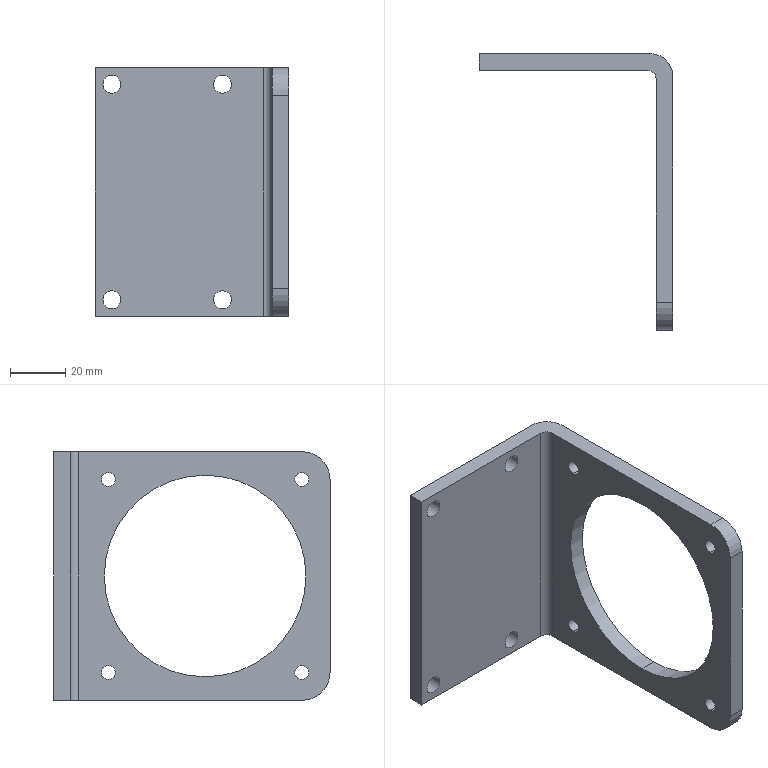Part | STEP file | X77-04015 | 1 solid | 30 faces | box 70 x 100 x 90 mm | volume 60860 mm3 | cylinder 22 | plane 8 | commonest cylinder face diameters 5 x8 6.5 x8 20 x2 73 x2 6 x1 16 x1
STEP:
#1=CARTESIAN_POINT('',(364.189,-105.641,7.5));
#2=VERTEX_POINT('',#1);
#3=CARTESIAN_POINT('',(364.189,-105.641,12.5));
#4=VERTEX_POINT('',#3);
#5=CARTESIAN_POINT('',(364.189,-105.641,10.));
#6=DIRECTION('',(-1.,0.,0.));
#7=DIRECTION('',(0.,0.,1.));
#8=AXIS2_PLACEMENT_3D('',#5,#6,#7);
#9=CIRCLE('',#8,2.5);
#10=EDGE_CURVE('',#2,#4,#9,.T.);
#11=ORIENTED_EDGE('',*,*,#10,.F.);
#12=CARTESIAN_POINT('',(358.189,-105.641,7.5));
#13=VERTEX_POINT('',#12);
#14=CARTESIAN_POINT('',(358.189,-105.641,7.5));
#15=DIRECTION('',(-1.,0.,0.));
#16=VECTOR('',#15,1000.);
#17=LINE('',#14,#16);
#18=EDGE_CURVE('',#2,#13,#17,.T.);
#19=ORIENTED_EDGE('',*,*,#18,.T.);
#20=CARTESIAN_POINT('',(358.189,-105.641,12.5));
#21=VERTEX_POINT('',#20);
#22=CARTESIAN_POINT('',(358.189,-105.641,10.));
#23=DIRECTION('',(-1.,0.,0.));
#24=DIRECTION('',(0.,0.,1.));
#25=AXIS2_PLACEMENT_3D('',#22,#23,#24);
#26=CIRCLE('',#25,2.5);
#27=EDGE_CURVE('',#13,#21,#26,.T.);
#28=ORIENTED_EDGE('',*,*,#27,.T.);
#29=CARTESIAN_POINT('',(358.189,-105.641,12.5));
#30=DIRECTION('',(-1.,0.,0.));
#31=VECTOR('',#30,1000.);
#32=LINE('',#29,#31);
#33=EDGE_CURVE('',#4,#21,#32,.T.);
#34=ORIENTED_EDGE('',*,*,#33,.F.);
#35=EDGE_LOOP('',(#11,#19,#28,#34));
#36=FACE_OUTER_BOUND('',#35,.T.);
#37=CARTESIAN_POINT('',(358.189,-105.641,10.));
#38=DIRECTION('',(-1.,0.,0.));
#39=DIRECTION('',(0.,0.,1.));
#40=AXIS2_PLACEMENT_3D('',#37,#38,#39);
#41=CYLINDRICAL_SURFACE('',#40,2.5);
#42=ADVANCED_FACE('',(#36),#41,.F.);
#43=CARTESIAN_POINT('',(364.189,-105.641,77.5));
#44=VERTEX_POINT('',#43);
#45=CARTESIAN_POINT('',(364.189,-105.641,82.5));
#46=VERTEX_POINT('',#45);
#47=CARTESIAN_POINT('',(364.189,-105.641,80.));
#48=DIRECTION('',(-1.,0.,0.));
#49=DIRECTION('',(0.,0.,1.));
#50=AXIS2_PLACEMENT_3D('',#47,#48,#49);
#51=CIRCLE('',#50,2.5);
#52=EDGE_CURVE('',#44,#46,#51,.T.);
#53=ORIENTED_EDGE('',*,*,#52,.F.);
#54=CARTESIAN_POINT('',(358.189,-105.641,77.5));
#55=VERTEX_POINT('',#54);
#56=CARTESIAN_POINT('',(358.189,-105.641,77.5));
#57=DIRECTION('',(-1.,0.,0.));
#58=VECTOR('',#57,1000.);
#59=LINE('',#56,#58);
#60=EDGE_CURVE('',#44,#55,#59,.T.);
#61=ORIENTED_EDGE('',*,*,#60,.T.);
#62=CARTESIAN_POINT('',(358.189,-105.641,82.5));
#63=VERTEX_POINT('',#62);
#64=CARTESIAN_POINT('',(358.189,-105.641,80.));
#65=DIRECTION('',(-1.,0.,0.));
#66=DIRECTION('',(0.,0.,1.));
#67=AXIS2_PLACEMENT_3D('',#64,#65,#66);
#68=CIRCLE('',#67,2.5);
#69=EDGE_CURVE('',#55,#63,#68,.T.);
#70=ORIENTED_EDGE('',*,*,#69,.T.);
#71=CARTESIAN_POINT('',(358.189,-105.641,82.5));
#72=DIRECTION('',(-1.,0.,0.));
#73=VECTOR('',#72,1000.);
#74=LINE('',#71,#73);
#75=EDGE_CURVE('',#46,#63,#74,.T.);
#76=ORIENTED_EDGE('',*,*,#75,.F.);
#77=EDGE_LOOP('',(#53,#61,#70,#76));
#78=FACE_OUTER_BOUND('',#77,.T.);
#79=CARTESIAN_POINT('',(358.189,-105.641,80.));
#80=DIRECTION('',(-1.,0.,0.));
#81=DIRECTION('',(0.,0.,1.));
#82=AXIS2_PLACEMENT_3D('',#79,#80,#81);
#83=CYLINDRICAL_SURFACE('',#82,2.5);
#84=ADVANCED_FACE('',(#78),#83,.F.);
#85=CARTESIAN_POINT('',(364.189,-35.641,77.5));
#86=VERTEX_POINT('',#85);
#87=CARTESIAN_POINT('',(364.189,-35.641,82.5));
#88=VERTEX_POINT('',#87);
#89=CARTESIAN_POINT('',(364.189,-35.641,80.));
#90=DIRECTION('',(-1.,0.,0.));
#91=DIRECTION('',(0.,0.,1.));
#92=AXIS2_PLACEMENT_3D('',#89,#90,#91);
#93=CIRCLE('',#92,2.5);
#94=EDGE_CURVE('',#86,#88,#93,.T.);
#95=ORIENTED_EDGE('',*,*,#94,.F.);
#96=CARTESIAN_POINT('',(358.189,-35.641,77.5));
#97=VERTEX_POINT('',#96);
#98=CARTESIAN_POINT('',(358.189,-35.641,77.5));
#99=DIRECTION('',(-1.,0.,0.));
#100=VECTOR('',#99,1000.);
#101=LINE('',#98,#100);
#102=EDGE_CURVE('',#86,#97,#101,.T.);
#103=ORIENTED_EDGE('',*,*,#102,.T.);
#104=CARTESIAN_POINT('',(358.189,-35.641,82.5));
#105=VERTEX_POINT('',#104);
#106=CARTESIAN_POINT('',(358.189,-35.641,80.));
#107=DIRECTION('',(-1.,0.,0.));
#108=DIRECTION('',(0.,0.,1.));
#109=AXIS2_PLACEMENT_3D('',#106,#107,#108);
#110=CIRCLE('',#109,2.5);
#111=EDGE_CURVE('',#97,#105,#110,.T.);
#112=ORIENTED_EDGE('',*,*,#111,.T.);
#113=CARTESIAN_POINT('',(358.189,-35.641,82.5));
#114=DIRECTION('',(-1.,0.,0.));
#115=VECTOR('',#114,1000.);
#116=LINE('',#113,#115);
#117=EDGE_CURVE('',#88,#105,#116,.T.);
#118=ORIENTED_EDGE('',*,*,#117,.F.);
#119=EDGE_LOOP('',(#95,#103,#112,#118));
#120=FACE_OUTER_BOUND('',#119,.T.);
#121=CARTESIAN_POINT('',(358.189,-35.641,80.));
#122=DIRECTION('',(-1.,0.,0.));
#123=DIRECTION('',(0.,0.,1.));
#124=AXIS2_PLACEMENT_3D('',#121,#122,#123);
#125=CYLINDRICAL_SURFACE('',#124,2.5);
#126=ADVANCED_FACE('',(#120),#125,.F.);
#127=CARTESIAN_POINT('',(364.189,-35.641,7.5));
#128=VERTEX_POINT('',#127);
#129=CARTESIAN_POINT('',(364.189,-35.641,12.5));
#130=VERTEX_POINT('',#129);
#131=CARTESIAN_POINT('',(364.189,-35.641,10.));
#132=DIRECTION('',(-1.,0.,0.));
#133=DIRECTION('',(0.,0.,1.));
#134=AXIS2_PLACEMENT_3D('',#131,#132,#133);
#135=CIRCLE('',#134,2.5);
#136=EDGE_CURVE('',#128,#130,#135,.T.);
#137=ORIENTED_EDGE('',*,*,#136,.F.);
#138=CARTESIAN_POINT('',(358.189,-35.641,7.5));
#139=VERTEX_POINT('',#138);
#140=CARTESIAN_POINT('',(358.189,-35.641,7.5));
#141=DIRECTION('',(-1.,0.,0.));
#142=VECTOR('',#141,1000.);
#143=LINE('',#140,#142);
#144=EDGE_CURVE('',#128,#139,#143,.T.);
#145=ORIENTED_EDGE('',*,*,#144,.T.);
#146=CARTESIAN_POINT('',(358.189,-35.641,12.5));
#147=VERTEX_POINT('',#146);
#148=CARTESIAN_POINT('',(358.189,-35.641,10.));
#149=DIRECTION('',(-1.,0.,0.));
#150=DIRECTION('',(0.,0.,1.));
#151=AXIS2_PLACEMENT_3D('',#148,#149,#150);
#152=CIRCLE('',#151,2.5);
#153=EDGE_CURVE('',#139,#147,#152,.T.);
#154=ORIENTED_EDGE('',*,*,#153,.T.);
#155=CARTESIAN_POINT('',(358.189,-35.641,12.5));
#156=DIRECTION('',(-1.,0.,0.));
#157=VECTOR('',#156,1000.);
#158=LINE('',#155,#157);
#159=EDGE_CURVE('',#130,#147,#158,.T.);
#160=ORIENTED_EDGE('',*,*,#159,.F.);
#161=EDGE_LOOP('',(#137,#145,#154,#160));
#162=FACE_OUTER_BOUND('',#161,.T.);
#163=CARTESIAN_POINT('',(358.189,-35.641,10.));
#164=DIRECTION('',(-1.,0.,0.));
#165=DIRECTION('',(0.,0.,1.));
#166=AXIS2_PLACEMENT_3D('',#163,#164,#165);
#167=CYLINDRICAL_SURFACE('',#166,2.5);
#168=ADVANCED_FACE('',(#162),#167,.F.);
#169=CARTESIAN_POINT('',(296.939,-15.891,6.));
#170=VERTEX_POINT('',#169);
#171=CARTESIAN_POINT('',(303.439,-15.891,6.));
#172=VERTEX_POINT('',#171);
#173=CARTESIAN_POINT('',(300.189,-15.891,6.));
#174=DIRECTION('',(0.,-1.,0.));
#175=DIRECTION('',(0.,0.,-1.));
#176=AXIS2_PLACEMENT_3D('',#173,#174,#175);
#177=CIRCLE('',#176,3.25);
#178=EDGE_CURVE('',#170,#172,#177,.T.);
#179=ORIENTED_EDGE('',*,*,#178,.F.);
#180=CARTESIAN_POINT('',(296.939,-21.891,6.));
#181=VERTEX_POINT('',#180);
#182=CARTESIAN_POINT('',(296.939,-11.891,6.));
#183=DIRECTION('',(0.,-1.,0.));
#184=VECTOR('',#183,1000.);
#185=LINE('',#182,#184);
#186=EDGE_CURVE('',#170,#181,#185,.T.);
#187=ORIENTED_EDGE('',*,*,#186,.T.);
#188=CARTESIAN_POINT('',(303.439,-21.891,6.));
#189=VERTEX_POINT('',#188);
#190=CARTESIAN_POINT('',(300.189,-21.891,6.));
#191=DIRECTION('',(0.,-1.,0.));
#192=DIRECTION('',(1.,0.,0.));
#193=AXIS2_PLACEMENT_3D('',#190,#191,#192);
#194=CIRCLE('',#193,3.25);
#195=EDGE_CURVE('',#181,#189,#194,.T.);
#196=ORIENTED_EDGE('',*,*,#195,.T.);
#197=CARTESIAN_POINT('',(303.439,-11.891,6.));
#198=DIRECTION('',(0.,-1.,0.));
#199=VECTOR('',#198,1000.);
#200=LINE('',#197,#199);
#201=EDGE_CURVE('',#172,#189,#200,.T.);
#202=ORIENTED_EDGE('',*,*,#201,.F.);
#203=EDGE_LOOP('',(#179,#187,#196,#202));
#204=FACE_OUTER_BOUND('',#203,.T.);
#205=CARTESIAN_POINT('',(300.189,-11.891,6.));
#206=DIRECTION('',(0.,-1.,0.));
#207=DIRECTION('',(1.,0.,0.));
#208=AXIS2_PLACEMENT_3D('',#205,#206,#207);
#209=CYLINDRICAL_SURFACE('',#208,3.25);
#210=ADVANCED_FACE('',(#204),#209,.F.);
#211=CARTESIAN_POINT('',(336.939,-15.891,6.));
#212=VERTEX_POINT('',#211);
#213=CARTESIAN_POINT('',(343.439,-15.891,6.));
#214=VERTEX_POINT('',#213);
#215=CARTESIAN_POINT('',(340.189,-15.891,6.));
#216=DIRECTION('',(0.,-1.,0.));
#217=DIRECTION('',(0.,0.,-1.));
#218=AXIS2_PLACEMENT_3D('',#215,#216,#217);
#219=CIRCLE('',#218,3.25);
#220=EDGE_CURVE('',#212,#214,#219,.T.);
#221=ORIENTED_EDGE('',*,*,#220,.F.);
#222=CARTESIAN_POINT('',(336.939,-21.891,6.));
#223=VERTEX_POINT('',#222);
#224=CARTESIAN_POINT('',(336.939,-11.891,6.));
#225=DIRECTION('',(0.,-1.,0.));
#226=VECTOR('',#225,1000.);
#227=LINE('',#224,#226);
#228=EDGE_CURVE('',#212,#223,#227,.T.);
#229=ORIENTED_EDGE('',*,*,#228,.T.);
#230=CARTESIAN_POINT('',(343.439,-21.891,6.));
#231=VERTEX_POINT('',#230);
#232=CARTESIAN_POINT('',(340.189,-21.891,6.));
#233=DIRECTION('',(0.,-1.,0.));
#234=DIRECTION('',(1.,0.,0.));
#235=AXIS2_PLACEMENT_3D('',#232,#233,#234);
#236=CIRCLE('',#235,3.25);
#237=EDGE_CURVE('',#223,#231,#236,.T.);
#238=ORIENTED_EDGE('',*,*,#237,.T.);
#239=CARTESIAN_POINT('',(343.439,-11.891,6.));
#240=DIRECTION('',(0.,-1.,0.));
#241=VECTOR('',#240,1000.);
#242=LINE('',#239,#241);
#243=EDGE_CURVE('',#214,#231,#242,.T.);
#244=ORIENTED_EDGE('',*,*,#243,.F.);
#245=EDGE_LOOP('',(#221,#229,#238,#244));
#246=FACE_OUTER_BOUND('',#245,.T.);
#247=CARTESIAN_POINT('',(340.189,-11.891,6.));
#248=DIRECTION('',(0.,-1.,0.));
#249=DIRECTION('',(1.,0.,0.));
#250=AXIS2_PLACEMENT_3D('',#247,#248,#249);
#251=CYLINDRICAL_SURFACE('',#250,3.25);
#252=ADVANCED_FACE('',(#246),#251,.F.);
#253=CARTESIAN_POINT('',(336.939,-15.891,84.));
#254=VERTEX_POINT('',#253);
#255=CARTESIAN_POINT('',(343.439,-15.891,84.));
#256=VERTEX_POINT('',#255);
#257=CARTESIAN_POINT('',(340.189,-15.891,84.));
#258=DIRECTION('',(0.,-1.,0.));
#259=DIRECTION('',(0.,0.,-1.));
#260=AXIS2_PLACEMENT_3D('',#257,#258,#259);
#261=CIRCLE('',#260,3.25);
#262=EDGE_CURVE('',#254,#256,#261,.T.);
#263=ORIENTED_EDGE('',*,*,#262,.F.);
#264=CARTESIAN_POINT('',(336.939,-21.891,84.));
#265=VERTEX_POINT('',#264);
#266=CARTESIAN_POINT('',(336.939,-11.891,84.));
#267=DIRECTION('',(0.,-1.,0.));
#268=VECTOR('',#267,1000.);
#269=LINE('',#266,#268);
#270=EDGE_CURVE('',#254,#265,#269,.T.);
#271=ORIENTED_EDGE('',*,*,#270,.T.);
#272=CARTESIAN_POINT('',(343.439,-21.891,84.));
#273=VERTEX_POINT('',#272);
#274=CARTESIAN_POINT('',(340.189,-21.891,84.));
#275=DIRECTION('',(0.,-1.,0.));
#276=DIRECTION('',(1.,0.,0.));
#277=AXIS2_PLACEMENT_3D('',#274,#275,#276);
#278=CIRCLE('',#277,3.25);
#279=EDGE_CURVE('',#265,#273,#278,.T.);
#280=ORIENTED_EDGE('',*,*,#279,.T.);
#281=CARTESIAN_POINT('',(343.439,-11.891,84.));
#282=DIRECTION('',(0.,-1.,0.));
#283=VECTOR('',#282,1000.);
#284=LINE('',#281,#283);
#285=EDGE_CURVE('',#256,#273,#284,.T.);
#286=ORIENTED_EDGE('',*,*,#285,.F.);
#287=EDGE_LOOP('',(#263,#271,#280,#286));
#288=FACE_OUTER_BOUND('',#287,.T.);
#289=CARTESIAN_POINT('',(340.189,-11.891,84.));
#290=DIRECTION('',(0.,-1.,0.));
#291=DIRECTION('',(1.,0.,0.));
#292=AXIS2_PLACEMENT_3D('',#289,#290,#291);
#293=CYLINDRICAL_SURFACE('',#292,3.25);
#294=ADVANCED_FACE('',(#288),#293,.F.);
#295=CARTESIAN_POINT('',(296.939,-15.891,84.));
#296=VERTEX_POINT('',#295);
#297=CARTESIAN_POINT('',(303.439,-15.891,84.));
#298=VERTEX_POINT('',#297);
#299=CARTESIAN_POINT('',(300.189,-15.891,84.));
#300=DIRECTION('',(0.,-1.,0.));
#301=DIRECTION('',(0.,0.,-1.));
#302=AXIS2_PLACEMENT_3D('',#299,#300,#301);
#303=CIRCLE('',#302,3.25);
#304=EDGE_CURVE('',#296,#298,#303,.T.);
#305=ORIENTED_EDGE('',*,*,#304,.F.);
#306=CARTESIAN_POINT('',(296.939,-21.891,84.));
#307=VERTEX_POINT('',#306);
#308=CARTESIAN_POINT('',(296.939,-11.891,84.));
#309=DIRECTION('',(0.,-1.,0.));
#310=VECTOR('',#309,1000.);
#311=LINE('',#308,#310);
#312=EDGE_CURVE('',#296,#307,#311,.T.);
#313=ORIENTED_EDGE('',*,*,#312,.T.);
#314=CARTESIAN_POINT('',(303.439,-21.891,84.));
#315=VERTEX_POINT('',#314);
#316=CARTESIAN_POINT('',(300.189,-21.891,84.));
#317=DIRECTION('',(0.,-1.,0.));
#318=DIRECTION('',(1.,0.,0.));
#319=AXIS2_PLACEMENT_3D('',#316,#317,#318);
#320=CIRCLE('',#319,3.25);
#321=EDGE_CURVE('',#307,#315,#320,.T.);
#322=ORIENTED_EDGE('',*,*,#321,.T.);
#323=CARTESIAN_POINT('',(303.439,-11.891,84.));
#324=DIRECTION('',(0.,-1.,0.));
#325=VECTOR('',#324,1000.);
#326=LINE('',#323,#325);
#327=EDGE_CURVE('',#298,#315,#326,.T.);
#328=ORIENTED_EDGE('',*,*,#327,.F.);
#329=EDGE_LOOP('',(#305,#313,#322,#328));
#330=FACE_OUTER_BOUND('',#329,.T.);
#331=CARTESIAN_POINT('',(300.189,-11.891,84.));
#332=DIRECTION('',(0.,-1.,0.));
#333=DIRECTION('',(1.,0.,0.));
#334=AXIS2_PLACEMENT_3D('',#331,#332,#333);
#335=CYLINDRICAL_SURFACE('',#334,3.25);
#336=ADVANCED_FACE('',(#330),#335,.F.);
#337=CARTESIAN_POINT('',(358.189,-70.641,81.5));
#338=VERTEX_POINT('',#337);
#339=CARTESIAN_POINT('',(358.189,-70.641,8.5));
#340=VERTEX_POINT('',#339);
#341=CARTESIAN_POINT('',(358.189,-70.641,45.));
#342=DIRECTION('',(1.,0.,0.));
#343=DIRECTION('',(0.,0.,-1.));
#344=AXIS2_PLACEMENT_3D('',#341,#342,#343);
#345=CIRCLE('',#344,36.5);
#346=EDGE_CURVE('',#338,#340,#345,.T.);
#347=ORIENTED_EDGE('',*,*,#346,.F.);
#348=CARTESIAN_POINT('',(364.189,-70.641,81.5));
#349=VERTEX_POINT('',#348);
#350=CARTESIAN_POINT('',(354.189,-70.641,81.5));
#351=DIRECTION('',(1.,0.,0.));
#352=VECTOR('',#351,1000.);
#353=LINE('',#350,#352);
#354=EDGE_CURVE('',#338,#349,#353,.T.);
#355=ORIENTED_EDGE('',*,*,#354,.T.);
#356=CARTESIAN_POINT('',(364.189,-70.641,8.5));
#357=VERTEX_POINT('',#356);
#358=CARTESIAN_POINT('',(364.189,-70.641,45.));
#359=DIRECTION('',(1.,0.,0.));
#360=DIRECTION('',(0.,0.,-1.));
#361=AXIS2_PLACEMENT_3D('',#358,#359,#360);
#362=CIRCLE('',#361,36.5);
#363=EDGE_CURVE('',#349,#357,#362,.T.);
#364=ORIENTED_EDGE('',*,*,#363,.T.);
#365=CARTESIAN_POINT('',(354.189,-70.641,8.5));
#366=DIRECTION('',(1.,0.,0.));
#367=VECTOR('',#366,1000.);
#368=LINE('',#365,#367);
#369=EDGE_CURVE('',#340,#357,#368,.T.);
#370=ORIENTED_EDGE('',*,*,#369,.F.);
#371=EDGE_LOOP('',(#347,#355,#364,#370));
#372=FACE_OUTER_BOUND('',#371,.T.);
#373=CARTESIAN_POINT('',(354.189,-70.641,45.));
#374=DIRECTION('',(1.,0.,0.));
#375=DIRECTION('',(0.,0.,-1.));
#376=AXIS2_PLACEMENT_3D('',#373,#374,#375);
#377=CYLINDRICAL_SURFACE('',#376,36.5);
#378=ADVANCED_FACE('',(#372),#377,.F.);
#379=CARTESIAN_POINT('',(358.189,-115.891,80.));
#380=VERTEX_POINT('',#379);
#381=CARTESIAN_POINT('',(358.189,-115.891,10.));
#382=VERTEX_POINT('',#381);
#383=CARTESIAN_POINT('',(358.189,-115.891,90.));
#384=DIRECTION('',(0.,0.,-1.));
#385=VECTOR('',#384,1000.);
#386=LINE('',#383,#385);
#387=EDGE_CURVE('',#380,#382,#386,.T.);
#388=ORIENTED_EDGE('',*,*,#387,.T.);
#389=CARTESIAN_POINT('',(364.189,-115.891,10.));
#390=VERTEX_POINT('',#389);
#391=CARTESIAN_POINT('',(364.189,-115.891,10.));
#392=DIRECTION('',(1.,0.,0.));
#393=VECTOR('',#392,1000.);
#394=LINE('',#391,#393);
#395=EDGE_CURVE('',#382,#390,#394,.T.);
#396=ORIENTED_EDGE('',*,*,#395,.T.);
#397=CARTESIAN_POINT('',(364.189,-115.891,80.));
#398=VERTEX_POINT('',#397);
#399=CARTESIAN_POINT('',(364.189,-115.891,90.));
#400=DIRECTION('',(0.,0.,-1.));
#401=VECTOR('',#400,1000.);
#402=LINE('',#399,#401);
#403=EDGE_CURVE('',#398,#390,#402,.T.);
#404=ORIENTED_EDGE('',*,*,#403,.F.);
#405=CARTESIAN_POINT('',(364.189,-115.891,80.));
#406=DIRECTION('',(-1.,0.,0.));
#407=VECTOR('',#406,1000.);
#408=LINE('',#405,#407);
#409=EDGE_CURVE('',#398,#380,#408,.T.);
#410=ORIENTED_EDGE('',*,*,#409,.T.);
#411=EDGE_LOOP('',(#388,#396,#404,#410));
#412=FACE_OUTER_BOUND('',#411,.T.);
#413=CARTESIAN_POINT('',(364.189,-115.891,90.));
#414=DIRECTION('',(0.,1.,0.));
#415=DIRECTION('',(0.,0.,1.));
#416=AXIS2_PLACEMENT_3D('',#413,#414,#415);
#417=PLANE('',#416);
#418=ADVANCED_FACE('',(#412),#417,.F.);
#419=CARTESIAN_POINT('',(364.189,-105.641,10.));
#420=DIRECTION('',(-1.,0.,0.));
#421=DIRECTION('',(0.,0.,1.));
#422=AXIS2_PLACEMENT_3D('',#419,#420,#421);
#423=CIRCLE('',#422,2.5);
#424=EDGE_CURVE('',#4,#2,#423,.T.);
#425=ORIENTED_EDGE('',*,*,#424,.T.);
#426=ORIENTED_EDGE('',*,*,#10,.T.);
#427=EDGE_LOOP('',(#425,#426));
#428=FACE_BOUND('',#427,.T.);
#429=CARTESIAN_POINT('',(364.189,-105.641,80.));
#430=DIRECTION('',(-1.,0.,0.));
#431=DIRECTION('',(0.,0.,1.));
#432=AXIS2_PLACEMENT_3D('',#429,#430,#431);
#433=CIRCLE('',#432,2.5);
#434=EDGE_CURVE('',#46,#44,#433,.T.);
#435=ORIENTED_EDGE('',*,*,#434,.T.);
#436=ORIENTED_EDGE('',*,*,#52,.T.);
#437=EDGE_LOOP('',(#435,#436));
#438=FACE_BOUND('',#437,.T.);
#439=CARTESIAN_POINT('',(364.189,-35.641,80.));
#440=DIRECTION('',(-1.,0.,0.));
#441=DIRECTION('',(0.,0.,1.));
#442=AXIS2_PLACEMENT_3D('',#439,#440,#441);
#443=CIRCLE('',#442,2.5);
#444=EDGE_CURVE('',#88,#86,#443,.T.);
#445=ORIENTED_EDGE('',*,*,#444,.T.);
#446=ORIENTED_EDGE('',*,*,#94,.T.);
#447=EDGE_LOOP('',(#445,#446));
#448=FACE_BOUND('',#447,.T.);
#449=CARTESIAN_POINT('',(364.189,-35.641,10.));
#450=DIRECTION('',(-1.,0.,0.));
#451=DIRECTION('',(0.,0.,1.));
#452=AXIS2_PLACEMENT_3D('',#449,#450,#451);
#453=CIRCLE('',#452,2.5);
#454=EDGE_CURVE('',#130,#128,#453,.T.);
#455=ORIENTED_EDGE('',*,*,#454,.T.);
#456=ORIENTED_EDGE('',*,*,#136,.T.);
#457=EDGE_LOOP('',(#455,#456));
#458=FACE_BOUND('',#457,.T.);
#459=CARTESIAN_POINT('',(364.189,-70.641,45.));
#460=DIRECTION('',(1.,0.,0.));
#461=DIRECTION('',(0.,0.,-1.));
#462=AXIS2_PLACEMENT_3D('',#459,#460,#461);
#463=CIRCLE('',#462,36.5);
#464=EDGE_CURVE('',#357,#349,#463,.T.);
#465=ORIENTED_EDGE('',*,*,#464,.F.);
#466=ORIENTED_EDGE('',*,*,#363,.F.);
#467=EDGE_LOOP('',(#465,#466));
#468=FACE_BOUND('',#467,.T.);
#469=ORIENTED_EDGE('',*,*,#403,.T.);
#470=CARTESIAN_POINT('',(364.189,-105.891,0.));
#471=VERTEX_POINT('',#470);
#472=CARTESIAN_POINT('',(364.189,-105.891,10.));
#473=DIRECTION('',(1.,0.,0.));
#474=DIRECTION('',(0.,0.,1.));
#475=AXIS2_PLACEMENT_3D('',#472,#473,#474);
#476=CIRCLE('',#475,10.);
#477=EDGE_CURVE('',#390,#471,#476,.T.);
#478=ORIENTED_EDGE('',*,*,#477,.T.);
#479=CARTESIAN_POINT('',(364.189,-23.891,0.));
#480=VERTEX_POINT('',#479);
#481=CARTESIAN_POINT('',(364.189,-23.891,0.));
#482=DIRECTION('',(0.,1.,0.));
#483=VECTOR('',#482,1000.);
#484=LINE('',#481,#483);
#485=EDGE_CURVE('',#471,#480,#484,.T.);
#486=ORIENTED_EDGE('',*,*,#485,.T.);
#487=CARTESIAN_POINT('',(364.189,-23.891,90.));
#488=VERTEX_POINT('',#487);
#489=CARTESIAN_POINT('',(364.189,-23.891,90.));
#490=DIRECTION('',(0.,0.,-1.));
#491=VECTOR('',#490,1000.);
#492=LINE('',#489,#491);
#493=EDGE_CURVE('',#488,#480,#492,.T.);
#494=ORIENTED_EDGE('',*,*,#493,.F.);
#495=CARTESIAN_POINT('',(364.189,-105.891,90.));
#496=VERTEX_POINT('',#495);
#497=CARTESIAN_POINT('',(364.189,-23.891,90.));
#498=DIRECTION('',(0.,1.,0.));
#499=VECTOR('',#498,1000.);
#500=LINE('',#497,#499);
#501=EDGE_CURVE('',#496,#488,#500,.T.);
#502=ORIENTED_EDGE('',*,*,#501,.F.);
#503=CARTESIAN_POINT('',(364.189,-105.891,80.));
#504=DIRECTION('',(1.,0.,0.));
#505=DIRECTION('',(0.,0.,1.));
#506=AXIS2_PLACEMENT_3D('',#503,#504,#505);
#507=CIRCLE('',#506,10.);
#508=EDGE_CURVE('',#496,#398,#507,.T.);
#509=ORIENTED_EDGE('',*,*,#508,.T.);
#510=EDGE_LOOP('',(#469,#478,#486,#494,#502,#509));
#511=FACE_OUTER_BOUND('',#510,.T.);
#512=CARTESIAN_POINT('',(364.189,-23.891,90.));
#513=DIRECTION('',(-1.,0.,0.));
#514=DIRECTION('',(0.,0.,1.));
#515=AXIS2_PLACEMENT_3D('',#512,#513,#514);
#516=PLANE('',#515);
#517=ADVANCED_FACE('',(#428,#438,#448,#458,#468,#511),#516,.F.);
#518=CARTESIAN_POINT('',(356.189,-15.891,0.));
#519=VERTEX_POINT('',#518);
#520=CARTESIAN_POINT('',(356.189,-23.891,0.));
#521=DIRECTION('',(0.,0.,1.));
#522=DIRECTION('',(-1.,0.,0.));
#523=AXIS2_PLACEMENT_3D('',#520,#521,#522);
#524=CIRCLE('',#523,8.);
#525=EDGE_CURVE('',#480,#519,#524,.T.);
#526=ORIENTED_EDGE('',*,*,#525,.T.);
#527=CARTESIAN_POINT('',(356.189,-15.891,90.));
#528=VERTEX_POINT('',#527);
#529=CARTESIAN_POINT('',(356.189,-15.891,90.));
#530=DIRECTION('',(0.,0.,-1.));
#531=VECTOR('',#530,1000.);
#532=LINE('',#529,#531);
#533=EDGE_CURVE('',#528,#519,#532,.T.);
#534=ORIENTED_EDGE('',*,*,#533,.F.);
#535=CARTESIAN_POINT('',(356.189,-23.891,90.));
#536=DIRECTION('',(0.,0.,1.));
#537=DIRECTION('',(-1.,0.,0.));
#538=AXIS2_PLACEMENT_3D('',#535,#536,#537);
#539=CIRCLE('',#538,8.);
#540=EDGE_CURVE('',#488,#528,#539,.T.);
#541=ORIENTED_EDGE('',*,*,#540,.F.);
#542=ORIENTED_EDGE('',*,*,#493,.T.);
#543=EDGE_LOOP('',(#526,#534,#541,#542));
#544=FACE_OUTER_BOUND('',#543,.T.);
#545=CARTESIAN_POINT('',(356.189,-23.891,90.));
#546=DIRECTION('',(0.,0.,-1.));
#547=DIRECTION('',(-1.,0.,0.));
#548=AXIS2_PLACEMENT_3D('',#545,#546,#547);
#549=CYLINDRICAL_SURFACE('',#548,8.);
#550=ADVANCED_FACE('',(#544),#549,.T.);
#551=CARTESIAN_POINT('',(300.189,-15.891,6.));
#552=DIRECTION('',(0.,-1.,0.));
#553=DIRECTION('',(0.,0.,-1.));
#554=AXIS2_PLACEMENT_3D('',#551,#552,#553);
#555=CIRCLE('',#554,3.25);
#556=EDGE_CURVE('',#172,#170,#555,.T.);
#557=ORIENTED_EDGE('',*,*,#556,.T.);
#558=ORIENTED_EDGE('',*,*,#178,.T.);
#559=EDGE_LOOP('',(#557,#558));
#560=FACE_BOUND('',#559,.T.);
#561=CARTESIAN_POINT('',(340.189,-15.891,6.));
#562=DIRECTION('',(0.,-1.,0.));
#563=DIRECTION('',(0.,0.,-1.));
#564=AXIS2_PLACEMENT_3D('',#561,#562,#563);
#565=CIRCLE('',#564,3.25);
#566=EDGE_CURVE('',#214,#212,#565,.T.);
#567=ORIENTED_EDGE('',*,*,#566,.T.);
#568=ORIENTED_EDGE('',*,*,#220,.T.);
#569=EDGE_LOOP('',(#567,#568));
#570=FACE_BOUND('',#569,.T.);
#571=CARTESIAN_POINT('',(340.189,-15.891,84.));
#572=DIRECTION('',(0.,-1.,0.));
#573=DIRECTION('',(0.,0.,-1.));
#574=AXIS2_PLACEMENT_3D('',#571,#572,#573);
#575=CIRCLE('',#574,3.25);
#576=EDGE_CURVE('',#256,#254,#575,.T.);
#577=ORIENTED_EDGE('',*,*,#576,.T.);
#578=ORIENTED_EDGE('',*,*,#262,.T.);
#579=EDGE_LOOP('',(#577,#578));
#580=FACE_BOUND('',#579,.T.);
#581=CARTESIAN_POINT('',(300.189,-15.891,84.));
#582=DIRECTION('',(0.,-1.,0.));
#583=DIRECTION('',(0.,0.,-1.));
#584=AXIS2_PLACEMENT_3D('',#581,#582,#583);
#585=CIRCLE('',#584,3.25);
#586=EDGE_CURVE('',#298,#296,#585,.T.);
#587=ORIENTED_EDGE('',*,*,#586,.T.);
#588=ORIENTED_EDGE('',*,*,#304,.T.);
#589=EDGE_LOOP('',(#587,#588));
#590=FACE_BOUND('',#589,.T.);
#591=CARTESIAN_POINT('',(294.189,-15.891,0.));
#592=VERTEX_POINT('',#591);
#593=CARTESIAN_POINT('',(294.189,-15.891,0.));
#594=DIRECTION('',(-1.,0.,0.));
#595=VECTOR('',#594,1000.);
#596=LINE('',#593,#595);
#597=EDGE_CURVE('',#519,#592,#596,.T.);
#598=ORIENTED_EDGE('',*,*,#597,.T.);
#599=CARTESIAN_POINT('',(294.189,-15.891,90.));
#600=VERTEX_POINT('',#599);
#601=CARTESIAN_POINT('',(294.189,-15.891,90.));
#602=DIRECTION('',(0.,0.,-1.));
#603=VECTOR('',#602,1000.);
#604=LINE('',#601,#603);
#605=EDGE_CURVE('',#600,#592,#604,.T.);
#606=ORIENTED_EDGE('',*,*,#605,.F.);
#607=CARTESIAN_POINT('',(294.189,-15.891,90.));
#608=DIRECTION('',(-1.,0.,0.));
#609=VECTOR('',#608,1000.);
#610=LINE('',#607,#609);
#611=EDGE_CURVE('',#528,#600,#610,.T.);
#612=ORIENTED_EDGE('',*,*,#611,.F.);
#613=ORIENTED_EDGE('',*,*,#533,.T.);
#614=EDGE_LOOP('',(#598,#606,#612,#613));
#615=FACE_OUTER_BOUND('',#614,.T.);
#616=CARTESIAN_POINT('',(294.189,-15.891,90.));
#617=DIRECTION('',(0.,-1.,0.));
#618=DIRECTION('',(0.,0.,-1.));
#619=AXIS2_PLACEMENT_3D('',#616,#617,#618);
#620=PLANE('',#619);
#621=ADVANCED_FACE('',(#560,#570,#580,#590,#615),#620,.F.);
#622=CARTESIAN_POINT('',(294.189,-21.891,0.));
#623=VERTEX_POINT('',#622);
#624=CARTESIAN_POINT('',(294.189,-21.891,0.));
#625=DIRECTION('',(0.,-1.,0.));
#626=VECTOR('',#625,1000.);
#627=LINE('',#624,#626);
#628=EDGE_CURVE('',#592,#623,#627,.T.);
#629=ORIENTED_EDGE('',*,*,#628,.T.);
#630=CARTESIAN_POINT('',(294.189,-21.891,90.));
#631=VERTEX_POINT('',#630);
#632=CARTESIAN_POINT('',(294.189,-21.891,90.));
#633=DIRECTION('',(0.,0.,-1.));
#634=VECTOR('',#633,1000.);
#635=LINE('',#632,#634);
#636=EDGE_CURVE('',#631,#623,#635,.T.);
#637=ORIENTED_EDGE('',*,*,#636,.F.);
#638=CARTESIAN_POINT('',(294.189,-21.891,90.));
#639=DIRECTION('',(0.,-1.,0.));
#640=VECTOR('',#639,1000.);
#641=LINE('',#638,#640);
#642=EDGE_CURVE('',#600,#631,#641,.T.);
#643=ORIENTED_EDGE('',*,*,#642,.F.);
#644=ORIENTED_EDGE('',*,*,#605,.T.);
#645=EDGE_LOOP('',(#629,#637,#643,#644));
#646=FACE_OUTER_BOUND('',#645,.T.);
#647=CARTESIAN_POINT('',(294.189,-21.891,90.));
#648=DIRECTION('',(1.,0.,0.));
#649=DIRECTION('',(0.,0.,-1.));
#650=AXIS2_PLACEMENT_3D('',#647,#648,#649);
#651=PLANE('',#650);
#652=ADVANCED_FACE('',(#646),#651,.F.);
#653=CARTESIAN_POINT('',(300.189,-21.891,6.));
#654=DIRECTION('',(0.,-1.,0.));
#655=DIRECTION('',(1.,0.,0.));
#656=AXIS2_PLACEMENT_3D('',#653,#654,#655);
#657=CIRCLE('',#656,3.25);
#658=EDGE_CURVE('',#189,#181,#657,.T.);
#659=ORIENTED_EDGE('',*,*,#658,.F.);
#660=ORIENTED_EDGE('',*,*,#195,.F.);
#661=EDGE_LOOP('',(#659,#660));
#662=FACE_BOUND('',#661,.T.);
#663=CARTESIAN_POINT('',(340.189,-21.891,6.));
#664=DIRECTION('',(0.,-1.,0.));
#665=DIRECTION('',(1.,0.,0.));
#666=AXIS2_PLACEMENT_3D('',#663,#664,#665);
#667=CIRCLE('',#666,3.25);
#668=EDGE_CURVE('',#231,#223,#667,.T.);
#669=ORIENTED_EDGE('',*,*,#668,.F.);
#670=ORIENTED_EDGE('',*,*,#237,.F.);
#671=EDGE_LOOP('',(#669,#670));
#672=FACE_BOUND('',#671,.T.);
#673=CARTESIAN_POINT('',(340.189,-21.891,84.));
#674=DIRECTION('',(0.,-1.,0.));
#675=DIRECTION('',(1.,0.,0.));
#676=AXIS2_PLACEMENT_3D('',#673,#674,#675);
#677=CIRCLE('',#676,3.25);
#678=EDGE_CURVE('',#273,#265,#677,.T.);
#679=ORIENTED_EDGE('',*,*,#678,.F.);
#680=ORIENTED_EDGE('',*,*,#279,.F.);
#681=EDGE_LOOP('',(#679,#680));
#682=FACE_BOUND('',#681,.T.);
#683=CARTESIAN_POINT('',(300.189,-21.891,84.));
#684=DIRECTION('',(0.,-1.,0.));
#685=DIRECTION('',(1.,0.,0.));
#686=AXIS2_PLACEMENT_3D('',#683,#684,#685);
#687=CIRCLE('',#686,3.25);
#688=EDGE_CURVE('',#315,#307,#687,.T.);
#689=ORIENTED_EDGE('',*,*,#688,.F.);
#690=ORIENTED_EDGE('',*,*,#321,.F.);
#691=EDGE_LOOP('',(#689,#690));
#692=FACE_BOUND('',#691,.T.);
#693=CARTESIAN_POINT('',(355.189,-21.891,0.));
#694=VERTEX_POINT('',#693);
#695=CARTESIAN_POINT('',(355.189,-21.891,0.));
#696=DIRECTION('',(1.,0.,0.));
#697=VECTOR('',#696,1000.);
#698=LINE('',#695,#697);
#699=EDGE_CURVE('',#623,#694,#698,.T.);
#700=ORIENTED_EDGE('',*,*,#699,.T.);
#701=CARTESIAN_POINT('',(355.189,-21.891,90.));
#702=VERTEX_POINT('',#701);
#703=CARTESIAN_POINT('',(355.189,-21.891,90.));
#704=DIRECTION('',(0.,0.,-1.));
#705=VECTOR('',#704,1000.);
#706=LINE('',#703,#705);
#707=EDGE_CURVE('',#702,#694,#706,.T.);
#708=ORIENTED_EDGE('',*,*,#707,.F.);
#709=CARTESIAN_POINT('',(355.189,-21.891,90.));
#710=DIRECTION('',(1.,0.,0.));
#711=VECTOR('',#710,1000.);
#712=LINE('',#709,#711);
#713=EDGE_CURVE('',#631,#702,#712,.T.);
#714=ORIENTED_EDGE('',*,*,#713,.F.);
#715=ORIENTED_EDGE('',*,*,#636,.T.);
#716=EDGE_LOOP('',(#700,#708,#714,#715));
#717=FACE_OUTER_BOUND('',#716,.T.);
#718=CARTESIAN_POINT('',(355.189,-21.891,90.));
#719=DIRECTION('',(0.,1.,0.));
#720=DIRECTION('',(-1.,0.,0.));
#721=AXIS2_PLACEMENT_3D('',#718,#719,#720);
#722=PLANE('',#721);
#723=ADVANCED_FACE('',(#662,#672,#682,#692,#717),#722,.F.);
#724=CARTESIAN_POINT('',(358.189,-24.891,0.));
#725=VERTEX_POINT('',#724);
#726=CARTESIAN_POINT('',(355.189,-24.891,0.));
#727=DIRECTION('',(0.,0.,-1.));
#728=DIRECTION('',(-1.,0.,0.));
#729=AXIS2_PLACEMENT_3D('',#726,#727,#728);
#730=CIRCLE('',#729,3.);
#731=EDGE_CURVE('',#694,#725,#730,.T.);
#732=ORIENTED_EDGE('',*,*,#731,.T.);
#733=CARTESIAN_POINT('',(358.189,-24.891,90.));
#734=VERTEX_POINT('',#733);
#735=CARTESIAN_POINT('',(358.189,-24.891,90.));
#736=DIRECTION('',(0.,0.,-1.));
#737=VECTOR('',#736,1000.);
#738=LINE('',#735,#737);
#739=EDGE_CURVE('',#734,#725,#738,.T.);
#740=ORIENTED_EDGE('',*,*,#739,.F.);
#741=CARTESIAN_POINT('',(355.189,-24.891,90.));
#742=DIRECTION('',(0.,0.,-1.));
#743=DIRECTION('',(-1.,0.,0.));
#744=AXIS2_PLACEMENT_3D('',#741,#742,#743);
#745=CIRCLE('',#744,3.);
#746=EDGE_CURVE('',#702,#734,#745,.T.);
#747=ORIENTED_EDGE('',*,*,#746,.F.);
#748=ORIENTED_EDGE('',*,*,#707,.T.);
#749=EDGE_LOOP('',(#732,#740,#747,#748));
#750=FACE_OUTER_BOUND('',#749,.T.);
#751=CARTESIAN_POINT('',(355.189,-24.891,90.));
#752=DIRECTION('',(0.,0.,-1.));
#753=DIRECTION('',(-1.,0.,0.));
#754=AXIS2_PLACEMENT_3D('',#751,#752,#753);
#755=CYLINDRICAL_SURFACE('',#754,3.);
#756=ADVANCED_FACE('',(#750),#755,.F.);
#757=CARTESIAN_POINT('',(358.189,-105.641,10.));
#758=DIRECTION('',(-1.,0.,0.));
#759=DIRECTION('',(0.,0.,1.));
#760=AXIS2_PLACEMENT_3D('',#757,#758,#759);
#761=CIRCLE('',#760,2.5);
#762=EDGE_CURVE('',#21,#13,#761,.T.);
#763=ORIENTED_EDGE('',*,*,#762,.F.);
#764=ORIENTED_EDGE('',*,*,#27,.F.);
#765=EDGE_LOOP('',(#763,#764));
#766=FACE_BOUND('',#765,.T.);
#767=CARTESIAN_POINT('',(358.189,-105.641,80.));
#768=DIRECTION('',(-1.,0.,0.));
#769=DIRECTION('',(0.,0.,1.));
#770=AXIS2_PLACEMENT_3D('',#767,#768,#769);
#771=CIRCLE('',#770,2.5);
#772=EDGE_CURVE('',#63,#55,#771,.T.);
#773=ORIENTED_EDGE('',*,*,#772,.F.);
#774=ORIENTED_EDGE('',*,*,#69,.F.);
#775=EDGE_LOOP('',(#773,#774));
#776=FACE_BOUND('',#775,.T.);
#777=CARTESIAN_POINT('',(358.189,-35.641,80.));
#778=DIRECTION('',(-1.,0.,0.));
#779=DIRECTION('',(0.,0.,1.));
#780=AXIS2_PLACEMENT_3D('',#777,#778,#779);
#781=CIRCLE('',#780,2.5);
#782=EDGE_CURVE('',#105,#97,#781,.T.);
#783=ORIENTED_EDGE('',*,*,#782,.F.);
#784=ORIENTED_EDGE('',*,*,#111,.F.);
#785=EDGE_LOOP('',(#783,#784));
#786=FACE_BOUND('',#785,.T.);
#787=CARTESIAN_POINT('',(358.189,-35.641,10.));
#788=DIRECTION('',(-1.,0.,0.));
#789=DIRECTION('',(0.,0.,1.));
#790=AXIS2_PLACEMENT_3D('',#787,#788,#789);
#791=CIRCLE('',#790,2.5);
#792=EDGE_CURVE('',#147,#139,#791,.T.);
#793=ORIENTED_EDGE('',*,*,#792,.F.);
#794=ORIENTED_EDGE('',*,*,#153,.F.);
#795=EDGE_LOOP('',(#793,#794));
#796=FACE_BOUND('',#795,.T.);
#797=CARTESIAN_POINT('',(358.189,-70.641,45.));
#798=DIRECTION('',(1.,0.,0.));
#799=DIRECTION('',(0.,0.,-1.));
#800=AXIS2_PLACEMENT_3D('',#797,#798,#799);
#801=CIRCLE('',#800,36.5);
#802=EDGE_CURVE('',#340,#338,#801,.T.);
#803=ORIENTED_EDGE('',*,*,#802,.T.);
#804=ORIENTED_EDGE('',*,*,#346,.T.);
#805=EDGE_LOOP('',(#803,#804));
#806=FACE_BOUND('',#805,.T.);
#807=CARTESIAN_POINT('',(358.189,-105.891,0.));
#808=VERTEX_POINT('',#807);
#809=CARTESIAN_POINT('',(358.189,-115.891,0.));
#810=DIRECTION('',(0.,-1.,0.));
#811=VECTOR('',#810,1000.);
#812=LINE('',#809,#811);
#813=EDGE_CURVE('',#725,#808,#812,.T.);
#814=ORIENTED_EDGE('',*,*,#813,.T.);
#815=CARTESIAN_POINT('',(358.189,-105.891,10.));
#816=DIRECTION('',(-1.,0.,0.));
#817=DIRECTION('',(0.,0.,-1.));
#818=AXIS2_PLACEMENT_3D('',#815,#816,#817);
#819=CIRCLE('',#818,10.);
#820=EDGE_CURVE('',#808,#382,#819,.T.);
#821=ORIENTED_EDGE('',*,*,#820,.T.);
#822=ORIENTED_EDGE('',*,*,#387,.F.);
#823=CARTESIAN_POINT('',(358.189,-105.891,90.));
#824=VERTEX_POINT('',#823);
#825=CARTESIAN_POINT('',(358.189,-105.891,80.));
#826=DIRECTION('',(-1.,0.,0.));
#827=DIRECTION('',(0.,0.,-1.));
#828=AXIS2_PLACEMENT_3D('',#825,#826,#827);
#829=CIRCLE('',#828,10.);
#830=EDGE_CURVE('',#380,#824,#829,.T.);
#831=ORIENTED_EDGE('',*,*,#830,.T.);
#832=CARTESIAN_POINT('',(358.189,-115.891,90.));
#833=DIRECTION('',(0.,-1.,0.));
#834=VECTOR('',#833,1000.);
#835=LINE('',#832,#834);
#836=EDGE_CURVE('',#734,#824,#835,.T.);
#837=ORIENTED_EDGE('',*,*,#836,.F.);
#838=ORIENTED_EDGE('',*,*,#739,.T.);
#839=EDGE_LOOP('',(#814,#821,#822,#831,#837,#838));
#840=FACE_OUTER_BOUND('',#839,.T.);
#841=CARTESIAN_POINT('',(358.189,-115.891,90.));
#842=DIRECTION('',(1.,0.,0.));
#843=DIRECTION('',(0.,0.,-1.));
#844=AXIS2_PLACEMENT_3D('',#841,#842,#843);
#845=PLANE('',#844);
#846=ADVANCED_FACE('',(#766,#776,#786,#796,#806,#840),#845,.F.);
#847=ORIENTED_EDGE('',*,*,#836,.T.);
#848=CARTESIAN_POINT('',(355.189,-105.891,90.));
#849=DIRECTION('',(1.,0.,0.));
#850=VECTOR('',#849,1000.);
#851=LINE('',#848,#850);
#852=EDGE_CURVE('',#824,#496,#851,.T.);
#853=ORIENTED_EDGE('',*,*,#852,.T.);
#854=ORIENTED_EDGE('',*,*,#501,.T.);
#855=ORIENTED_EDGE('',*,*,#540,.T.);
#856=ORIENTED_EDGE('',*,*,#611,.T.);
#857=ORIENTED_EDGE('',*,*,#642,.T.);
#858=ORIENTED_EDGE('',*,*,#713,.T.);
#859=ORIENTED_EDGE('',*,*,#746,.T.);
#860=EDGE_LOOP('',(#847,#853,#854,#855,#856,#857,#858,#859));
#861=FACE_OUTER_BOUND('',#860,.T.);
#862=CARTESIAN_POINT('',(355.189,-24.891,90.));
#863=DIRECTION('',(0.,0.,-1.));
#864=DIRECTION('',(-1.,0.,0.));
#865=AXIS2_PLACEMENT_3D('',#862,#863,#864);
#866=PLANE('',#865);
#867=ADVANCED_FACE('',(#861),#866,.F.);
#868=ORIENTED_EDGE('',*,*,#485,.F.);
#869=CARTESIAN_POINT('',(358.189,-105.891,0.));
#870=DIRECTION('',(-1.,0.,0.));
#871=VECTOR('',#870,1000.);
#872=LINE('',#869,#871);
#873=EDGE_CURVE('',#471,#808,#872,.T.);
#874=ORIENTED_EDGE('',*,*,#873,.T.);
#875=ORIENTED_EDGE('',*,*,#813,.F.);
#876=ORIENTED_EDGE('',*,*,#731,.F.);
#877=ORIENTED_EDGE('',*,*,#699,.F.);
#878=ORIENTED_EDGE('',*,*,#628,.F.);
#879=ORIENTED_EDGE('',*,*,#597,.F.);
#880=ORIENTED_EDGE('',*,*,#525,.F.);
#881=EDGE_LOOP('',(#868,#874,#875,#876,#877,#878,#879,#880));
#882=FACE_OUTER_BOUND('',#881,.T.);
#883=CARTESIAN_POINT('',(355.189,-24.891,0.));
#884=DIRECTION('',(0.,0.,-1.));
#885=DIRECTION('',(-1.,0.,0.));
#886=AXIS2_PLACEMENT_3D('',#883,#884,#885);
#887=PLANE('',#886);
#888=ADVANCED_FACE('',(#882),#887,.T.);
#889=ORIENTED_EDGE('',*,*,#354,.F.);
#890=ORIENTED_EDGE('',*,*,#802,.F.);
#891=ORIENTED_EDGE('',*,*,#369,.T.);
#892=ORIENTED_EDGE('',*,*,#464,.T.);
#893=EDGE_LOOP('',(#889,#890,#891,#892));
#894=FACE_OUTER_BOUND('',#893,.T.);
#895=CARTESIAN_POINT('',(354.189,-70.641,45.));
#896=DIRECTION('',(1.,0.,0.));
#897=DIRECTION('',(0.,0.,-1.));
#898=AXIS2_PLACEMENT_3D('',#895,#896,#897);
#899=CYLINDRICAL_SURFACE('',#898,36.5);
#900=ADVANCED_FACE('',(#894),#899,.F.);
#901=ORIENTED_EDGE('',*,*,#820,.F.);
#902=ORIENTED_EDGE('',*,*,#873,.F.);
#903=ORIENTED_EDGE('',*,*,#477,.F.);
#904=ORIENTED_EDGE('',*,*,#395,.F.);
#905=EDGE_LOOP('',(#901,#902,#903,#904));
#906=FACE_OUTER_BOUND('',#905,.T.);
#907=CARTESIAN_POINT('',(364.189,-105.891,10.));
#908=DIRECTION('',(-1.,0.,0.));
#909=DIRECTION('',(0.,0.,1.));
#910=AXIS2_PLACEMENT_3D('',#907,#908,#909);
#911=CYLINDRICAL_SURFACE('',#910,10.);
#912=ADVANCED_FACE('',(#906),#911,.T.);
#913=ORIENTED_EDGE('',*,*,#830,.F.);
#914=ORIENTED_EDGE('',*,*,#409,.F.);
#915=ORIENTED_EDGE('',*,*,#508,.F.);
#916=ORIENTED_EDGE('',*,*,#852,.F.);
#917=EDGE_LOOP('',(#913,#914,#915,#916));
#918=FACE_OUTER_BOUND('',#917,.T.);
#919=CARTESIAN_POINT('',(355.189,-105.891,80.));
#920=DIRECTION('',(1.,0.,0.));
#921=DIRECTION('',(0.,0.,-1.));
#922=AXIS2_PLACEMENT_3D('',#919,#920,#921);
#923=CYLINDRICAL_SURFACE('',#922,10.);
#924=ADVANCED_FACE('',(#918),#923,.T.);
#925=ORIENTED_EDGE('',*,*,#312,.F.);
#926=ORIENTED_EDGE('',*,*,#586,.F.);
#927=ORIENTED_EDGE('',*,*,#327,.T.);
#928=ORIENTED_EDGE('',*,*,#688,.T.);
#929=EDGE_LOOP('',(#925,#926,#927,#928));
#930=FACE_OUTER_BOUND('',#929,.T.);
#931=CARTESIAN_POINT('',(300.189,-11.891,84.));
#932=DIRECTION('',(0.,-1.,0.));
#933=DIRECTION('',(1.,0.,0.));
#934=AXIS2_PLACEMENT_3D('',#931,#932,#933);
#935=CYLINDRICAL_SURFACE('',#934,3.25);
#936=ADVANCED_FACE('',(#930),#935,.F.);
#937=ORIENTED_EDGE('',*,*,#270,.F.);
#938=ORIENTED_EDGE('',*,*,#576,.F.);
#939=ORIENTED_EDGE('',*,*,#285,.T.);
#940=ORIENTED_EDGE('',*,*,#678,.T.);
#941=EDGE_LOOP('',(#937,#938,#939,#940));
#942=FACE_OUTER_BOUND('',#941,.T.);
#943=CARTESIAN_POINT('',(340.189,-11.891,84.));
#944=DIRECTION('',(0.,-1.,0.));
#945=DIRECTION('',(1.,0.,0.));
#946=AXIS2_PLACEMENT_3D('',#943,#944,#945);
#947=CYLINDRICAL_SURFACE('',#946,3.25);
#948=ADVANCED_FACE('',(#942),#947,.F.);
#949=ORIENTED_EDGE('',*,*,#228,.F.);
#950=ORIENTED_EDGE('',*,*,#566,.F.);
#951=ORIENTED_EDGE('',*,*,#243,.T.);
#952=ORIENTED_EDGE('',*,*,#668,.T.);
#953=EDGE_LOOP('',(#949,#950,#951,#952));
#954=FACE_OUTER_BOUND('',#953,.T.);
#955=CARTESIAN_POINT('',(340.189,-11.891,6.));
#956=DIRECTION('',(0.,-1.,0.));
#957=DIRECTION('',(1.,0.,0.));
#958=AXIS2_PLACEMENT_3D('',#955,#956,#957);
#959=CYLINDRICAL_SURFACE('',#958,3.25);
#960=ADVANCED_FACE('',(#954),#959,.F.);
#961=ORIENTED_EDGE('',*,*,#186,.F.);
#962=ORIENTED_EDGE('',*,*,#556,.F.);
#963=ORIENTED_EDGE('',*,*,#201,.T.);
#964=ORIENTED_EDGE('',*,*,#658,.T.);
#965=EDGE_LOOP('',(#961,#962,#963,#964));
#966=FACE_OUTER_BOUND('',#965,.T.);
#967=CARTESIAN_POINT('',(300.189,-11.891,6.));
#968=DIRECTION('',(0.,-1.,0.));
#969=DIRECTION('',(1.,0.,0.));
#970=AXIS2_PLACEMENT_3D('',#967,#968,#969);
#971=CYLINDRICAL_SURFACE('',#970,3.25);
#972=ADVANCED_FACE('',(#966),#971,.F.);
#973=ORIENTED_EDGE('',*,*,#144,.F.);
#974=ORIENTED_EDGE('',*,*,#454,.F.);
#975=ORIENTED_EDGE('',*,*,#159,.T.);
#976=ORIENTED_EDGE('',*,*,#792,.T.);
#977=EDGE_LOOP('',(#973,#974,#975,#976));
#978=FACE_OUTER_BOUND('',#977,.T.);
#979=CARTESIAN_POINT('',(358.189,-35.641,10.));
#980=DIRECTION('',(-1.,0.,0.));
#981=DIRECTION('',(0.,0.,1.));
#982=AXIS2_PLACEMENT_3D('',#979,#980,#981);
#983=CYLINDRICAL_SURFACE('',#982,2.5);
#984=ADVANCED_FACE('',(#978),#983,.F.);
#985=ORIENTED_EDGE('',*,*,#102,.F.);
#986=ORIENTED_EDGE('',*,*,#444,.F.);
#987=ORIENTED_EDGE('',*,*,#117,.T.);
#988=ORIENTED_EDGE('',*,*,#782,.T.);
#989=EDGE_LOOP('',(#985,#986,#987,#988));
#990=FACE_OUTER_BOUND('',#989,.T.);
#991=CARTESIAN_POINT('',(358.189,-35.641,80.));
#992=DIRECTION('',(-1.,0.,0.));
#993=DIRECTION('',(0.,0.,1.));
#994=AXIS2_PLACEMENT_3D('',#991,#992,#993);
#995=CYLINDRICAL_SURFACE('',#994,2.5);
#996=ADVANCED_FACE('',(#990),#995,.F.);
#997=ORIENTED_EDGE('',*,*,#60,.F.);
#998=ORIENTED_EDGE('',*,*,#434,.F.);
#999=ORIENTED_EDGE('',*,*,#75,.T.);
#1000=ORIENTED_EDGE('',*,*,#772,.T.);
#1001=EDGE_LOOP('',(#997,#998,#999,#1000));
#1002=FACE_OUTER_BOUND('',#1001,.T.);
#1003=CARTESIAN_POINT('',(358.189,-105.641,80.));
#1004=DIRECTION('',(-1.,0.,0.));
#1005=DIRECTION('',(0.,0.,1.));
#1006=AXIS2_PLACEMENT_3D('',#1003,#1004,#1005);
#1007=CYLINDRICAL_SURFACE('',#1006,2.5);
#1008=ADVANCED_FACE('',(#1002),#1007,.F.);
#1009=ORIENTED_EDGE('',*,*,#18,.F.);
#1010=ORIENTED_EDGE('',*,*,#424,.F.);
#1011=ORIENTED_EDGE('',*,*,#33,.T.);
#1012=ORIENTED_EDGE('',*,*,#762,.T.);
#1013=EDGE_LOOP('',(#1009,#1010,#1011,#1012));
#1014=FACE_OUTER_BOUND('',#1013,.T.);
#1015=CARTESIAN_POINT('',(358.189,-105.641,10.));
#1016=DIRECTION('',(-1.,0.,0.));
#1017=DIRECTION('',(0.,0.,1.));
#1018=AXIS2_PLACEMENT_3D('',#1015,#1016,#1017);
#1019=CYLINDRICAL_SURFACE('',#1018,2.5);
#1020=ADVANCED_FACE('',(#1014),#1019,.F.);
#1021=CLOSED_SHELL('',(#42,#84,#126,#168,#210,#252,#294,#336,#378,#418,#517,#550,#621,#652,#723,#756,#846,#867,#888,#900,#912,#924,#936,#948,#960,#972,#984,#996,#1008,#1020));
#1022=MANIFOLD_SOLID_BREP('',#1021);
#1023=CARTESIAN_POINT('',(0.,0.,0.));
#1024=DIRECTION('',(0.,0.,1.));
#1025=DIRECTION('',(1.,0.,0.));
#1026=AXIS2_PLACEMENT_3D('',#1023,#1024,#1025);
#1027=(LENGTH_UNIT()NAMED_UNIT(*)SI_UNIT(.MILLI.,.METRE.));
#1028=UNCERTAINTY_MEASURE_WITH_UNIT(LENGTH_MEASURE(0.00001),#1027,'','');
#1029=(NAMED_UNIT(*)PLANE_ANGLE_UNIT()SI_UNIT($,.RADIAN.));
#1030=(NAMED_UNIT(*)SI_UNIT($,.STERADIAN.)SOLID_ANGLE_UNIT());
#1031=(GEOMETRIC_REPRESENTATION_CONTEXT(3)GLOBAL_UNCERTAINTY_ASSIGNED_CONTEXT((#1028))GLOBAL_UNIT_ASSIGNED_CONTEXT((#1027,#1029,#1030))REPRESENTATION_CONTEXT('',''));
#1032=ADVANCED_BREP_SHAPE_REPRESENTATION('',(#1022,#1026),#1031);